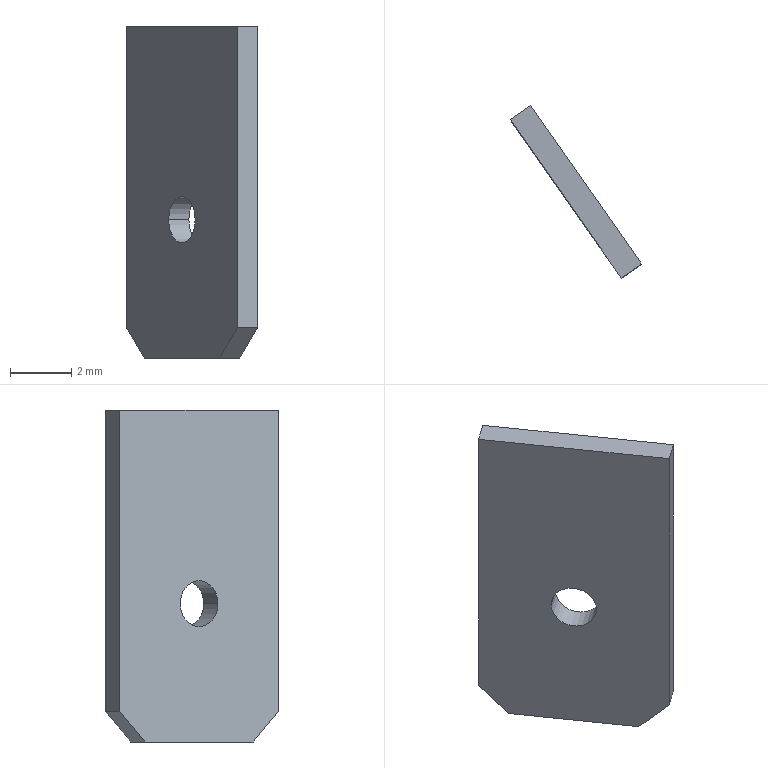Part | STEP file | JAIREIPAN_146_2_1 | 1 solid | 10 faces | box 4.269 x 5.62 x 10.8 mm | volume 52.218 mm3 | plane 8 | cylinder 2 | commonest cylinder face diameters 1.5 x2
STEP:
#1=CARTESIAN_POINT('',(0.,0.,0.));
#2=DIRECTION('',(0.,0.,1.));
#3=DIRECTION('',(1.,0.,0.));
#4=AXIS2_PLACEMENT_3D('',#1,#2,#3);
#5=CARTESIAN_POINT('',(35.899,24.221,-9.3));
#6=VERTEX_POINT('',#5);
#7=CARTESIAN_POINT('',(35.244,23.763,-9.3));
#8=VERTEX_POINT('',#7);
#9=CARTESIAN_POINT('',(35.899,24.221,-9.3));
#10=DIRECTION('',(-0.8192,-0.5736,0.));
#11=VECTOR('',#10,0.8);
#12=LINE('',#9,#11);
#13=EDGE_CURVE('',#6,#8,#12,.T.);
#14=ORIENTED_EDGE('',*,*,#13,.F.);
#15=CARTESIAN_POINT('',(35.039,25.45,-9.3));
#16=VERTEX_POINT('',#15);
#17=CARTESIAN_POINT('',(35.469,24.836,-9.3));
#18=DIRECTION('',(0.8192,0.5736,0.));
#19=DIRECTION('',(-0.5736,0.8192,0.));
#20=AXIS2_PLACEMENT_3D('',#17,#18,#19);
#21=CIRCLE('',#20,0.75);
#22=EDGE_CURVE('',#16,#6,#21,.T.);
#23=ORIENTED_EDGE('',*,*,#22,.F.);
#24=CARTESIAN_POINT('',(34.384,24.991,-9.3));
#25=VERTEX_POINT('',#24);
#26=CARTESIAN_POINT('',(35.039,25.45,-9.3));
#27=DIRECTION('',(-0.8192,-0.5736,0.));
#28=VECTOR('',#27,0.8);
#29=LINE('',#26,#28);
#30=EDGE_CURVE('',#16,#25,#29,.T.);
#31=ORIENTED_EDGE('',*,*,#30,.T.);
#32=CARTESIAN_POINT('',(34.814,24.377,-9.3));
#33=DIRECTION('',(-0.8192,-0.5736,0.));
#34=DIRECTION('',(0.5736,-0.8192,0.));
#35=AXIS2_PLACEMENT_3D('',#32,#33,#34);
#36=CIRCLE('',#35,0.75);
#37=EDGE_CURVE('',#8,#25,#36,.T.);
#38=ORIENTED_EDGE('',*,*,#37,.F.);
#39=EDGE_LOOP('',(#14,#23,#31,#38));
#40=FACE_OUTER_BOUND('',#39,.F.);
#41=CARTESIAN_POINT('',(35.469,24.836,-9.3));
#42=DIRECTION('',(0.8192,0.5736,0.));
#43=DIRECTION('',(0.5736,-0.8192,0.));
#44=AXIS2_PLACEMENT_3D('',#41,#42,#43);
#45=CYLINDRICAL_SURFACE('',#44,0.75);
#46=ADVANCED_FACE('',(#40),#45,.F.);
#47=ORIENTED_EDGE('',*,*,#13,.T.);
#48=CARTESIAN_POINT('',(34.814,24.377,-9.3));
#49=DIRECTION('',(-0.8192,-0.5736,0.));
#50=DIRECTION('',(-0.5736,0.8192,0.));
#51=AXIS2_PLACEMENT_3D('',#48,#49,#50);
#52=CIRCLE('',#51,0.75);
#53=EDGE_CURVE('',#25,#8,#52,.T.);
#54=ORIENTED_EDGE('',*,*,#53,.F.);
#55=ORIENTED_EDGE('',*,*,#30,.F.);
#56=CARTESIAN_POINT('',(35.469,24.836,-9.3));
#57=DIRECTION('',(0.8192,0.5736,0.));
#58=DIRECTION('',(0.5736,-0.8192,0.));
#59=AXIS2_PLACEMENT_3D('',#56,#57,#58);
#60=CIRCLE('',#59,0.75);
#61=EDGE_CURVE('',#6,#16,#60,.T.);
#62=ORIENTED_EDGE('',*,*,#61,.F.);
#63=EDGE_LOOP('',(#47,#54,#55,#62));
#64=FACE_OUTER_BOUND('',#63,.F.);
#65=CARTESIAN_POINT('',(35.469,24.836,-9.3));
#66=DIRECTION('',(0.8192,0.5736,0.));
#67=DIRECTION('',(0.5736,-0.8192,0.));
#68=AXIS2_PLACEMENT_3D('',#65,#66,#67);
#69=CYLINDRICAL_SURFACE('',#68,0.75);
#70=ADVANCED_FACE('',(#64),#69,.F.);
#71=CARTESIAN_POINT('',(36.621,21.797,-12.8));
#72=VERTEX_POINT('',#71);
#73=CARTESIAN_POINT('',(36.047,22.616,-13.8));
#74=VERTEX_POINT('',#73);
#75=CARTESIAN_POINT('',(36.621,21.797,-12.8));
#76=DIRECTION('',(-0.4056,0.5792,-0.7071));
#77=VECTOR('',#76,1.414);
#78=LINE('',#75,#77);
#79=EDGE_CURVE('',#72,#74,#78,.T.);
#80=ORIENTED_EDGE('',*,*,#79,.T.);
#81=CARTESIAN_POINT('',(33.581,26.138,-13.8));
#82=VERTEX_POINT('',#81);
#83=CARTESIAN_POINT('',(33.581,26.138,-13.8));
#84=DIRECTION('',(0.5736,-0.8192,0.));
#85=VECTOR('',#84,4.3);
#86=LINE('',#83,#85);
#87=EDGE_CURVE('',#82,#74,#86,.T.);
#88=ORIENTED_EDGE('',*,*,#87,.F.);
#89=CARTESIAN_POINT('',(33.007,26.957,-12.8));
#90=VERTEX_POINT('',#89);
#91=CARTESIAN_POINT('',(33.581,26.138,-13.8));
#92=DIRECTION('',(-0.4056,0.5792,0.7071));
#93=VECTOR('',#92,1.414);
#94=LINE('',#91,#93);
#95=EDGE_CURVE('',#82,#90,#94,.T.);
#96=ORIENTED_EDGE('',*,*,#95,.T.);
#97=CARTESIAN_POINT('',(33.007,26.957,-3.));
#98=VERTEX_POINT('',#97);
#99=CARTESIAN_POINT('',(33.007,26.957,-3.));
#100=DIRECTION('',(0.,0.,-1.));
#101=VECTOR('',#100,9.8);
#102=LINE('',#99,#101);
#103=EDGE_CURVE('',#98,#90,#102,.T.);
#104=ORIENTED_EDGE('',*,*,#103,.F.);
#105=CARTESIAN_POINT('',(36.621,21.797,-3.));
#106=VERTEX_POINT('',#105);
#107=CARTESIAN_POINT('',(36.621,21.797,-3.));
#108=DIRECTION('',(-0.5736,0.8192,0.));
#109=VECTOR('',#108,6.3);
#110=LINE('',#107,#109);
#111=EDGE_CURVE('',#106,#98,#110,.T.);
#112=ORIENTED_EDGE('',*,*,#111,.F.);
#113=CARTESIAN_POINT('',(36.621,21.797,-3.));
#114=DIRECTION('',(0.,0.,-1.));
#115=VECTOR('',#114,9.8);
#116=LINE('',#113,#115);
#117=EDGE_CURVE('',#106,#72,#116,.T.);
#118=ORIENTED_EDGE('',*,*,#117,.T.);
#119=EDGE_LOOP('',(#80,#88,#96,#104,#112,#118));
#120=FACE_OUTER_BOUND('',#119,.F.);
#121=ORIENTED_EDGE('',*,*,#53,.T.);
#122=ORIENTED_EDGE('',*,*,#37,.T.);
#123=EDGE_LOOP('',(#121,#122));
#124=FACE_BOUND('',#123,.F.);
#125=CARTESIAN_POINT('',(36.621,21.797,-3.));
#126=DIRECTION('',(-0.8192,-0.5736,0.));
#127=DIRECTION('',(-0.5736,0.8192,0.));
#128=AXIS2_PLACEMENT_3D('',#125,#126,#127);
#129=PLANE('',#128);
#130=ADVANCED_FACE('',(#120,#124),#129,.T.);
#131=ORIENTED_EDGE('',*,*,#79,.F.);
#132=CARTESIAN_POINT('',(37.276,22.256,-12.8));
#133=VERTEX_POINT('',#132);
#134=CARTESIAN_POINT('',(37.276,22.256,-12.8));
#135=DIRECTION('',(-0.8192,-0.5736,0.));
#136=VECTOR('',#135,0.8);
#137=LINE('',#134,#136);
#138=EDGE_CURVE('',#133,#72,#137,.T.);
#139=ORIENTED_EDGE('',*,*,#138,.F.);
#140=CARTESIAN_POINT('',(36.702,23.075,-13.8));
#141=VERTEX_POINT('',#140);
#142=CARTESIAN_POINT('',(36.702,23.075,-13.8));
#143=DIRECTION('',(0.4056,-0.5792,0.7071));
#144=VECTOR('',#143,1.414);
#145=LINE('',#142,#144);
#146=EDGE_CURVE('',#141,#133,#145,.T.);
#147=ORIENTED_EDGE('',*,*,#146,.F.);
#148=CARTESIAN_POINT('',(36.047,22.616,-13.8));
#149=DIRECTION('',(0.8192,0.5736,0.));
#150=VECTOR('',#149,0.8);
#151=LINE('',#148,#150);
#152=EDGE_CURVE('',#74,#141,#151,.T.);
#153=ORIENTED_EDGE('',*,*,#152,.F.);
#154=EDGE_LOOP('',(#131,#139,#147,#153));
#155=FACE_OUTER_BOUND('',#154,.F.);
#156=CARTESIAN_POINT('',(36.662,22.436,-13.3));
#157=DIRECTION('',(0.4056,-0.5792,-0.7071));
#158=DIRECTION('',(0.4056,-0.5792,0.7071));
#159=AXIS2_PLACEMENT_3D('',#156,#157,#158);
#160=PLANE('',#159);
#161=ADVANCED_FACE('',(#155),#160,.T.);
#162=ORIENTED_EDGE('',*,*,#138,.T.);
#163=ORIENTED_EDGE('',*,*,#117,.F.);
#164=CARTESIAN_POINT('',(37.276,22.256,-3.));
#165=VERTEX_POINT('',#164);
#166=CARTESIAN_POINT('',(37.276,22.256,-3.));
#167=DIRECTION('',(-0.8192,-0.5736,0.));
#168=VECTOR('',#167,0.8);
#169=LINE('',#166,#168);
#170=EDGE_CURVE('',#165,#106,#169,.T.);
#171=ORIENTED_EDGE('',*,*,#170,.F.);
#172=CARTESIAN_POINT('',(37.276,22.256,-3.));
#173=DIRECTION('',(0.,0.,-1.));
#174=VECTOR('',#173,9.8);
#175=LINE('',#172,#174);
#176=EDGE_CURVE('',#165,#133,#175,.T.);
#177=ORIENTED_EDGE('',*,*,#176,.T.);
#178=EDGE_LOOP('',(#162,#163,#171,#177));
#179=FACE_OUTER_BOUND('',#178,.F.);
#180=CARTESIAN_POINT('',(37.276,22.256,-3.));
#181=DIRECTION('',(0.5736,-0.8192,0.));
#182=DIRECTION('',(-0.8192,-0.5736,0.));
#183=AXIS2_PLACEMENT_3D('',#180,#181,#182);
#184=PLANE('',#183);
#185=ADVANCED_FACE('',(#179),#184,.T.);
#186=CARTESIAN_POINT('',(33.663,27.416,-3.));
#187=VERTEX_POINT('',#186);
#188=CARTESIAN_POINT('',(33.007,26.957,-3.));
#189=DIRECTION('',(0.8192,0.5736,0.));
#190=VECTOR('',#189,0.8);
#191=LINE('',#188,#190);
#192=EDGE_CURVE('',#98,#187,#191,.T.);
#193=ORIENTED_EDGE('',*,*,#192,.T.);
#194=CARTESIAN_POINT('',(33.663,27.416,-3.));
#195=DIRECTION('',(0.5736,-0.8192,0.));
#196=VECTOR('',#195,6.3);
#197=LINE('',#194,#196);
#198=EDGE_CURVE('',#187,#165,#197,.T.);
#199=ORIENTED_EDGE('',*,*,#198,.T.);
#200=ORIENTED_EDGE('',*,*,#170,.T.);
#201=ORIENTED_EDGE('',*,*,#111,.T.);
#202=EDGE_LOOP('',(#193,#199,#200,#201));
#203=FACE_OUTER_BOUND('',#202,.F.);
#204=CARTESIAN_POINT('',(0.,0.,-3.));
#205=DIRECTION('',(0.,0.,-1.));
#206=DIRECTION('',(1.,0.,0.));
#207=AXIS2_PLACEMENT_3D('',#204,#205,#206);
#208=PLANE('',#207);
#209=ADVANCED_FACE('',(#203),#208,.F.);
#210=CARTESIAN_POINT('',(33.663,27.416,-12.8));
#211=VERTEX_POINT('',#210);
#212=CARTESIAN_POINT('',(33.007,26.957,-12.8));
#213=DIRECTION('',(0.8192,0.5736,0.));
#214=VECTOR('',#213,0.8);
#215=LINE('',#212,#214);
#216=EDGE_CURVE('',#90,#211,#215,.T.);
#217=ORIENTED_EDGE('',*,*,#216,.T.);
#218=CARTESIAN_POINT('',(33.663,27.416,-3.));
#219=DIRECTION('',(0.,0.,-1.));
#220=VECTOR('',#219,9.8);
#221=LINE('',#218,#220);
#222=EDGE_CURVE('',#187,#211,#221,.T.);
#223=ORIENTED_EDGE('',*,*,#222,.F.);
#224=ORIENTED_EDGE('',*,*,#192,.F.);
#225=ORIENTED_EDGE('',*,*,#103,.T.);
#226=EDGE_LOOP('',(#217,#223,#224,#225));
#227=FACE_OUTER_BOUND('',#226,.F.);
#228=CARTESIAN_POINT('',(33.007,26.957,-3.));
#229=DIRECTION('',(-0.5736,0.8192,0.));
#230=DIRECTION('',(0.8192,0.5736,0.));
#231=AXIS2_PLACEMENT_3D('',#228,#229,#230);
#232=PLANE('',#231);
#233=ADVANCED_FACE('',(#227),#232,.T.);
#234=CARTESIAN_POINT('',(34.236,26.597,-13.8));
#235=VERTEX_POINT('',#234);
#236=CARTESIAN_POINT('',(33.663,27.416,-12.8));
#237=DIRECTION('',(0.4056,-0.5792,-0.7071));
#238=VECTOR('',#237,1.414);
#239=LINE('',#236,#238);
#240=EDGE_CURVE('',#211,#235,#239,.T.);
#241=ORIENTED_EDGE('',*,*,#240,.F.);
#242=ORIENTED_EDGE('',*,*,#216,.F.);
#243=ORIENTED_EDGE('',*,*,#95,.F.);
#244=CARTESIAN_POINT('',(34.236,26.597,-13.8));
#245=DIRECTION('',(-0.8192,-0.5736,0.));
#246=VECTOR('',#245,0.8);
#247=LINE('',#244,#246);
#248=EDGE_CURVE('',#235,#82,#247,.T.);
#249=ORIENTED_EDGE('',*,*,#248,.F.);
#250=EDGE_LOOP('',(#241,#242,#243,#249));
#251=FACE_OUTER_BOUND('',#250,.F.);
#252=CARTESIAN_POINT('',(33.622,26.777,-13.3));
#253=DIRECTION('',(-0.4056,0.5792,-0.7071));
#254=DIRECTION('',(-0.4056,0.5792,0.7071));
#255=AXIS2_PLACEMENT_3D('',#252,#253,#254);
#256=PLANE('',#255);
#257=ADVANCED_FACE('',(#251),#256,.T.);
#258=ORIENTED_EDGE('',*,*,#146,.T.);
#259=ORIENTED_EDGE('',*,*,#176,.F.);
#260=ORIENTED_EDGE('',*,*,#198,.F.);
#261=ORIENTED_EDGE('',*,*,#222,.T.);
#262=ORIENTED_EDGE('',*,*,#240,.T.);
#263=CARTESIAN_POINT('',(36.702,23.075,-13.8));
#264=DIRECTION('',(-0.5736,0.8192,0.));
#265=VECTOR('',#264,4.3);
#266=LINE('',#263,#265);
#267=EDGE_CURVE('',#141,#235,#266,.T.);
#268=ORIENTED_EDGE('',*,*,#267,.F.);
#269=EDGE_LOOP('',(#258,#259,#260,#261,#262,#268));
#270=FACE_OUTER_BOUND('',#269,.F.);
#271=ORIENTED_EDGE('',*,*,#61,.T.);
#272=ORIENTED_EDGE('',*,*,#22,.T.);
#273=EDGE_LOOP('',(#271,#272));
#274=FACE_BOUND('',#273,.F.);
#275=CARTESIAN_POINT('',(33.663,27.416,-3.));
#276=DIRECTION('',(0.8192,0.5736,0.));
#277=DIRECTION('',(0.5736,-0.8192,0.));
#278=AXIS2_PLACEMENT_3D('',#275,#276,#277);
#279=PLANE('',#278);
#280=ADVANCED_FACE('',(#270,#274),#279,.T.);
#281=ORIENTED_EDGE('',*,*,#152,.T.);
#282=ORIENTED_EDGE('',*,*,#267,.T.);
#283=ORIENTED_EDGE('',*,*,#248,.T.);
#284=ORIENTED_EDGE('',*,*,#87,.T.);
#285=EDGE_LOOP('',(#281,#282,#283,#284));
#286=FACE_OUTER_BOUND('',#285,.F.);
#287=CARTESIAN_POINT('',(0.,0.,-13.8));
#288=DIRECTION('',(0.,0.,-1.));
#289=DIRECTION('',(0.,-1.,0.));
#290=AXIS2_PLACEMENT_3D('',#287,#288,#289);
#291=PLANE('',#290);
#292=ADVANCED_FACE('',(#286),#291,.T.);
#293=CLOSED_SHELL('',(#46,#70,#130,#161,#185,#209,#233,#257,#280,#292));
#294=MANIFOLD_SOLID_BREP('',#293);
#295=(LENGTH_UNIT()NAMED_UNIT(*)SI_UNIT(.MILLI.,.METRE.));
#296=UNCERTAINTY_MEASURE_WITH_UNIT(LENGTH_MEASURE(0.00129),#295,'','');
#297=(NAMED_UNIT(*)PLANE_ANGLE_UNIT()SI_UNIT($,.RADIAN.));
#298=PLANE_ANGLE_MEASURE_WITH_UNIT(PLANE_ANGLE_MEASURE(0.01745),#297);
#299=(CONVERSION_BASED_UNIT('DEGREE',#298)NAMED_UNIT(*)PLANE_ANGLE_UNIT());
#300=(NAMED_UNIT(*)SI_UNIT($,.STERADIAN.)SOLID_ANGLE_UNIT());
#301=(GEOMETRIC_REPRESENTATION_CONTEXT(3)GLOBAL_UNCERTAINTY_ASSIGNED_CONTEXT((#296))GLOBAL_UNIT_ASSIGNED_CONTEXT((#295,#299,#300))REPRESENTATION_CONTEXT('',''));
#302=ADVANCED_BREP_SHAPE_REPRESENTATION('',(#4,#294),#301);